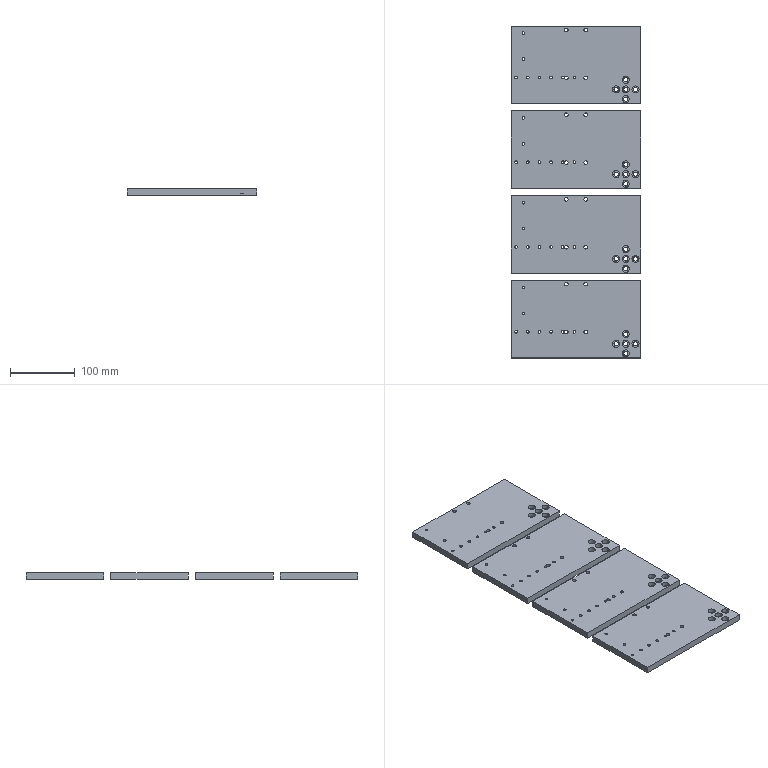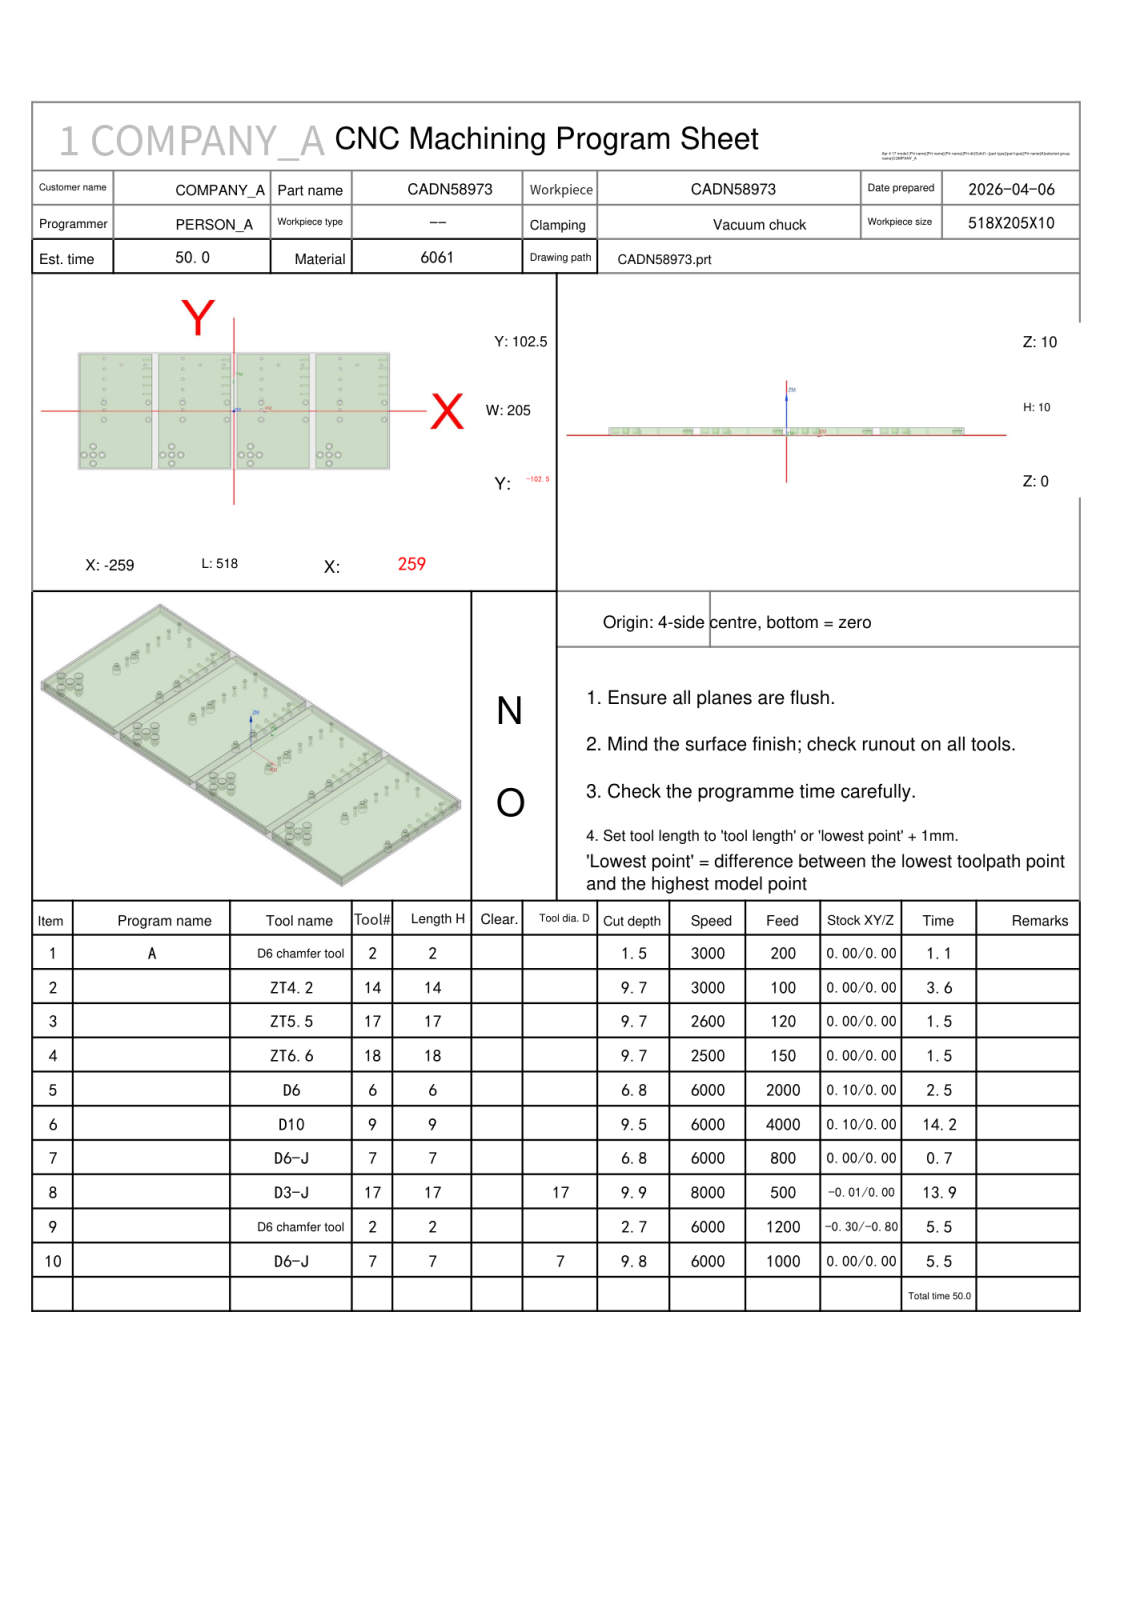NC program | NX | posted by the shop | part box 200 x 513 x 10 mm
Lines 1768 to 2551 of 10035:
N8 T17 M06
(D3-J  D=3. R=0. H=17 ce=-0.01 di=0.00)
G00 G90 G54 X-216.146 Y1.994 M03 S8000
G43 H17 Z30.
M08
Z10.5
G01 X-216.074 Y1.972 Z10.496 F500.
X-215.926 Z10.488
X-215.757 Y2.024 Z10.479
X-215.613 Y2.128 Z10.47
X-215.509 Y2.272 Z10.46
X-215.457 Y2.441 Z10.451
Y2.589 Z10.443
X-215.509 Y2.758 Z10.434
X-215.613 Y2.902 Z10.425
X-215.757 Y3.006 Z10.416
X-215.926 Y3.058 Z10.406
X-216.074 Z10.398
X-216.235 Y3.01 Z10.39
X-216.375 Y2.915 Z10.381
X-216.478 Y2.782 Z10.372
X-216.537 Y2.624 Z10.363
X-216.543 Y2.441 Z10.354
X-216.491 Y2.272 Z10.344
X-216.387 Y2.128 Z10.335
X-216.243 Y2.024 Z10.326
X-216.074 Y1.972 Z10.316
X-215.926 Z10.309
X-215.757 Y2.024 Z10.299
X-215.613 Y2.128 Z10.29
X-215.509 Y2.272 Z10.281
X-215.457 Y2.441 Z10.271
Y2.589 Z10.264
X-215.509 Y2.758 Z10.254
X-215.613 Y2.902 Z10.245
X-215.757 Y3.006 Z10.236
X-215.926 Y3.058 Z10.227
X-216.074 Z10.219
X-216.235 Y3.01 Z10.21
X-216.375 Y2.915 Z10.201
X-216.478 Y2.782 Z10.192
X-216.537 Y2.624 Z10.184
X-216.543 Y2.441 Z10.174
X-216.491 Y2.272 Z10.165
X-216.387 Y2.128 Z10.155
X-216.243 Y2.024 Z10.146
X-216.074 Y1.972 Z10.137
X-215.926 Z10.129
X-215.757 Y2.024 Z10.12
X-215.613 Y2.128 Z10.11
X-215.509 Y2.272 Z10.101
X-215.457 Y2.441 Z10.092
Y2.589 Z10.084
X-215.509 Y2.758 Z10.075
X-215.613 Y2.902 Z10.066
X-215.757 Y3.006 Z10.056
X-215.926 Y3.058 Z10.047
X-216.074 Z10.039
X-216.235 Y3.01 Z10.03
X-216.375 Y2.915 Z10.022
X-216.478 Y2.782 Z10.013
X-216.537 Y2.624 Z10.004
X-216.542 Y2.55 Z10.
G41 D17
X-216.577 Y2.515
G03 X-216. Y1.938 Z9.925 I.577 J0.0
X-215.423 Y2.515 Z9.851 I0.0 J.577
X-216. Y3.092 Z9.776 I-.577 J0.0
X-216.577 Y2.515 Z9.702 I0.0 J-.577
X-216. Y1.938 Z9.627 I.577 J0.0
X-215.423 Y2.515 Z9.552 I0.0 J.577
X-216. Y3.092 Z9.478 I-.577 J0.0
X-216.577 Y2.515 Z9.403 I0.0 J-.577
X-216. Y1.938 Z9.328 I.577 J0.0
X-215.423 Y2.515 Z9.254 I0.0 J.577
X-216. Y3.092 Z9.179 I-.577 J0.0
X-216.577 Y2.515 Z9.105 I0.0 J-.577
X-216. Y1.938 Z9.03 I.577 J0.0
X-215.423 Y2.515 Z8.955 I0.0 J.577
X-216. Y3.092 Z8.881 I-.577 J0.0
X-216.577 Y2.515 Z8.806 I0.0 J-.577
X-216. Y1.938 Z8.731 I.577 J0.0
X-215.423 Y2.515 Z8.657 I0.0 J.577
X-216. Y3.092 Z8.582 I-.577 J0.0
X-216.577 Y2.515 Z8.508 I0.0 J-.577
X-216. Y1.938 Z8.433 I.577 J0.0
X-215.423 Y2.515 Z8.358 I0.0 J.577
X-216. Y3.092 Z8.284 I-.577 J0.0
X-216.577 Y2.515 Z8.209 I0.0 J-.577
X-216. Y1.938 Z8.134 I.577 J0.0
X-215.423 Y2.515 Z8.06 I0.0 J.577
X-216. Y3.092 Z7.985 I-.577 J0.0
X-216.577 Y2.515 Z7.911 I0.0 J-.577
X-216. Y1.938 Z7.836 I.577 J0.0
X-215.423 Y2.515 Z7.761 I0.0 J.577
X-216. Y3.092 Z7.687 I-.577 J0.0
X-216.577 Y2.515 Z7.612 I0.0 J-.577
X-216. Y1.938 Z7.538 I.577 J0.0
X-215.423 Y2.515 Z7.463 I0.0 J.577
X-216. Y3.092 Z7.388 I-.577 J0.0
X-216.577 Y2.515 Z7.314 I0.0 J-.577
X-216. Y1.938 Z7.239 I.577 J0.0
X-215.423 Y2.515 Z7.164 I0.0 J.577
X-216. Y3.092 Z7.09 I-.577 J0.0
X-216.577 Y2.515 Z7.015 I0.0 J-.577
X-216. Y1.938 Z6.941 I.577 J0.0
X-215.423 Y2.515 Z6.866 I0.0 J.577
X-216. Y3.092 Z6.791 I-.577 J0.0
X-216.577 Y2.515 Z6.717 I0.0 J-.577
X-216. Y1.938 Z6.642 I.577 J0.0
X-215.423 Y2.515 Z6.567 I0.0 J.577
X-216. Y3.092 Z6.493 I-.577 J0.0
X-216.577 Y2.515 Z6.418 I0.0 J-.577
X-216. Y1.938 Z6.344 I.577 J0.0
X-215.423 Y2.515 Z6.269 I0.0 J.577
X-216. Y3.092 Z6.194 I-.577 J0.0
X-216.577 Y2.515 Z6.12 I0.0 J-.577
X-216. Y1.938 Z6.045 I.577 J0.0
X-215.423 Y2.515 Z5.97 I0.0 J.577
X-216. Y3.092 Z5.896 I-.577 J0.0
X-216.577 Y2.515 Z5.821 I0.0 J-.577
X-216. Y1.938 Z5.747 I.577 J0.0
X-215.423 Y2.515 Z5.672 I0.0 J.577
X-216. Y3.092 Z5.597 I-.577 J0.0
X-216.577 Y2.515 Z5.523 I0.0 J-.577
X-216. Y1.938 Z5.448 I.577 J0.0
X-215.423 Y2.515 Z5.373 I0.0 J.577
X-216. Y3.092 Z5.299 I-.577 J0.0
X-216.577 Y2.515 Z5.224 I0.0 J-.577
X-216. Y1.938 Z5.15 I.577 J0.0
X-215.423 Y2.515 Z5.075 I0.0 J.577
X-216. Y3.092 Z5. I-.577 J0.0
X-216.577 Y2.515 Z4.926 I0.0 J-.577
X-216. Y1.938 Z4.851 I.577 J0.0
X-215.423 Y2.515 Z4.777 I0.0 J.577
X-216. Y3.092 Z4.702 I-.577 J0.0
X-216.577 Y2.515 Z4.627 I0.0 J-.577
X-216. Y1.938 Z4.553 I.577 J0.0
X-215.423 Y2.515 Z4.478 I0.0 J.577
X-216. Y3.092 Z4.403 I-.577 J0.0
X-216.577 Y2.515 Z4.329 I0.0 J-.577
X-216. Y1.938 Z4.254 I.577 J0.0
X-215.423 Y2.515 Z4.18 I0.0 J.577
X-216. Y3.092 Z4.105 I-.577 J0.0
X-216.577 Y2.515 Z4.03 I0.0 J-.577
X-216. Y1.938 Z3.956 I.577 J0.0
X-215.423 Y2.515 Z3.881 I0.0 J.577
X-216. Y3.092 Z3.806 I-.577 J0.0
X-216.577 Y2.515 Z3.732 I0.0 J-.577
X-216. Y1.938 Z3.657 I.577 J0.0
X-215.423 Y2.515 Z3.583 I0.0 J.577
X-216. Y3.092 Z3.508 I-.577 J0.0
X-216.577 Y2.515 Z3.433 I0.0 J-.577
X-216. Y1.938 Z3.359 I.577 J0.0
X-215.423 Y2.515 Z3.284 I0.0 J.577
X-216. Y3.092 Z3.209 I-.577 J0.0
X-216.577 Y2.515 Z3.135 I0.0 J-.577
X-216. Y1.938 Z3.06 I.577 J0.0
X-215.423 Y2.515 Z2.986 I0.0 J.577
X-216. Y3.092 Z2.911 I-.577 J0.0
X-216.577 Y2.515 Z2.836 I0.0 J-.577
X-216. Y1.938 Z2.762 I.577 J0.0
X-215.423 Y2.515 Z2.687 I0.0 J.577
X-216. Y3.092 Z2.613 I-.577 J0.0
X-216.577 Y2.515 Z2.538 I0.0 J-.577
X-216. Y1.938 Z2.463 I.577 J0.0
X-215.423 Y2.515 Z2.389 I0.0 J.577
X-216. Y3.092 Z2.314 I-.577 J0.0
X-216.577 Y2.515 Z2.239 I0.0 J-.577
X-216. Y1.938 Z2.165 I.577 J0.0
X-215.423 Y2.515 Z2.09 I0.0 J.577
X-216. Y3.092 Z2.016 I-.577 J0.0
X-216.577 Y2.515 Z1.941 I0.0 J-.577
X-216. Y1.938 Z1.866 I.577 J0.0
X-215.423 Y2.515 Z1.792 I0.0 J.577
X-216. Y3.092 Z1.717 I-.577 J0.0
X-216.577 Y2.515 Z1.642 I0.0 J-.577
X-216. Y1.938 Z1.568 I.577 J0.0
X-215.423 Y2.515 Z1.493 I0.0 J.577
X-216. Y3.092 Z1.419 I-.577 J0.0
X-216.577 Y2.515 Z1.344 I0.0 J-.577
X-216. Y1.938 Z1.269 I.577 J0.0
X-215.423 Y2.515 Z1.195 I0.0 J.577
X-216. Y3.092 Z1.12 I-.577 J0.0
X-216.577 Y2.515 Z1.045 I0.0 J-.577
X-216. Y1.938 Z.971 I.577 J0.0
X-215.423 Y2.515 Z.896 I0.0 J.577
X-216. Y3.092 Z.822 I-.577 J0.0
X-216.577 Y2.515 Z.747 I0.0 J-.577
X-216. Y1.938 Z.672 I.577 J0.0
X-215.423 Y2.515 Z.598 I0.0 J.577
X-216. Y3.092 Z.523 I-.577 J0.0
X-216.577 Y2.515 Z.448 I0.0 J-.577
X-216. Y1.938 Z.374 I.577 J0.0
X-215.423 Y2.515 Z.299 I0.0 J.577
X-216. Y3.092 Z.225 I-.577 J0.0
X-216.577 Y2.515 Z.15 I0.0 J-.577
X-216. Y1.938 I.577 J0.0
X-215.423 Y2.515 I0.0 J.577
X-216. Y3.092 I-.577 J0.0
X-216.577 Y2.515 I0.0 J-.577
X-216.444 Y2.146 I.577 J0.0
G01 X-216.424 Y2.127
X-216.396 Y2.124
X-216.373 Y2.14
G40 X-216.335 Y2.172
Z1.15
G00 Z30.
X-216.144 Y37.994
Z10.5
G01 X-216.074 Y37.972 Z10.496
X-215.926 Z10.488
X-215.757 Y38.024 Z10.479
X-215.613 Y38.128 Z10.47
X-215.509 Y38.272 Z10.461
X-215.457 Y38.441 Z10.451
Y38.589 Z10.444
X-215.481 Y38.692 Z10.438
X-215.525 Y38.788 Z10.432
X-215.615 Y38.905 Z10.425
X-215.758 Y39.007 Z10.416
X-215.926 Y39.058 Z10.406
X-216.074 Z10.399
X-216.235 Y39.01 Z10.39
X-216.375 Y38.915 Z10.381
X-216.478 Y38.782 Z10.372
X-216.537 Y38.624 Z10.363
X-216.543 Y38.441 Z10.354
X-216.491 Y38.272 Z10.344
X-216.387 Y38.128 Z10.335
X-216.243 Y38.024 Z10.326
X-216.074 Y37.972 Z10.316
X-215.926 Z10.309
X-215.757 Y38.024 Z10.299
X-215.613 Y38.128 Z10.29
X-215.509 Y38.272 Z10.281
X-215.457 Y38.441 Z10.272
Y38.589 Z10.264
X-215.481 Y38.692 Z10.258
X-215.525 Y38.788 Z10.253
X-215.615 Y38.905 Z10.245
X-215.758 Y39.007 Z10.236
X-215.926 Y39.058 Z10.227
X-216.074 Z10.219
X-216.235 Y39.01 Z10.21
X-216.375 Y38.915 Z10.201
X-216.478 Y38.782 Z10.192
X-216.537 Y38.624 Z10.184
X-216.543 Y38.441 Z10.174
X-216.491 Y38.272 Z10.165
X-216.387 Y38.128 Z10.155
X-216.243 Y38.024 Z10.146
X-216.074 Y37.972 Z10.137
X-215.926 Z10.129
X-215.757 Y38.024 Z10.12
X-215.613 Y38.128 Z10.11
X-215.509 Y38.272 Z10.101
X-215.457 Y38.441 Z10.092
Y38.589 Z10.084
X-215.481 Y38.692 Z10.079
X-215.525 Y38.788 Z10.073
X-215.615 Y38.905 Z10.065
X-215.758 Y39.007 Z10.056
X-215.926 Y39.058 Z10.047
X-216.074 Z10.039
X-216.235 Y39.01 Z10.03
X-216.375 Y38.915 Z10.022
X-216.478 Y38.782 Z10.013
X-216.537 Y38.624 Z10.004
X-216.542 Y38.55 Z10.
G41 D17
X-216.577 Y38.515
G03 X-216. Y37.938 Z9.925 I.577 J0.0
X-215.423 Y38.515 Z9.851 I0.0 J.577
X-215.543 Y38.867 Z9.82 I-.577 J0.0
X-216. Y39.092 Z9.776 I-.457 J-.352
X-216.577 Y38.515 Z9.702 I0.0 J-.577
X-216. Y37.938 Z9.627 I.577 J0.0
X-215.423 Y38.515 Z9.552 I0.0 J.577
X-215.543 Y38.867 Z9.521 I-.577 J0.0
X-216. Y39.092 Z9.478 I-.457 J-.352
X-216.577 Y38.515 Z9.403 I0.0 J-.577
X-216. Y37.938 Z9.328 I.577 J0.0
X-215.423 Y38.515 Z9.254 I0.0 J.577
X-215.543 Y38.867 Z9.223 I-.577 J0.0
X-216. Y39.092 Z9.179 I-.457 J-.352
X-216.577 Y38.515 Z9.105 I0.0 J-.577
X-216. Y37.938 Z9.03 I.577 J0.0
X-215.423 Y38.515 Z8.955 I0.0 J.577
X-215.543 Y38.867 Z8.924 I-.577 J0.0
X-216. Y39.092 Z8.881 I-.457 J-.352
X-216.577 Y38.515 Z8.806 I0.0 J-.577
X-216. Y37.938 Z8.731 I.577 J0.0
X-215.423 Y38.515 Z8.657 I0.0 J.577
X-215.543 Y38.867 Z8.626 I-.577 J0.0
X-216. Y39.092 Z8.582 I-.457 J-.352
X-216.577 Y38.515 Z8.508 I0.0 J-.577
X-216. Y37.938 Z8.433 I.577 J0.0
X-215.423 Y38.515 Z8.358 I0.0 J.577
X-215.543 Y38.867 Z8.327 I-.577 J0.0
X-216. Y39.092 Z8.284 I-.457 J-.352
X-216.577 Y38.515 Z8.209 I0.0 J-.577
X-216. Y37.938 Z8.134 I.577 J0.0
X-215.423 Y38.515 Z8.06 I0.0 J.577
X-215.543 Y38.867 Z8.029 I-.577 J0.0
X-216. Y39.092 Z7.985 I-.457 J-.352
X-216.577 Y38.515 Z7.911 I0.0 J-.577
X-216. Y37.938 Z7.836 I.577 J0.0
X-215.423 Y38.515 Z7.761 I0.0 J.577
X-215.543 Y38.867 Z7.73 I-.577 J0.0
X-216. Y39.092 Z7.687 I-.457 J-.352
X-216.577 Y38.515 Z7.612 I0.0 J-.577
X-216. Y37.938 Z7.538 I.577 J0.0
X-215.423 Y38.515 Z7.463 I0.0 J.577
X-215.543 Y38.867 Z7.432 I-.577 J0.0
X-216. Y39.092 Z7.388 I-.457 J-.352
X-216.577 Y38.515 Z7.314 I0.0 J-.577
X-216. Y37.938 Z7.239 I.577 J0.0
X-215.423 Y38.515 Z7.164 I0.0 J.577
X-215.543 Y38.867 Z7.133 I-.577 J0.0
X-216. Y39.092 Z7.09 I-.457 J-.352
X-216.577 Y38.515 Z7.015 I0.0 J-.577
X-216. Y37.938 Z6.941 I.577 J0.0
X-215.423 Y38.515 Z6.866 I0.0 J.577
X-215.543 Y38.867 Z6.835 I-.577 J0.0
X-216. Y39.092 Z6.791 I-.457 J-.352
X-216.577 Y38.515 Z6.717 I0.0 J-.577
X-216. Y37.938 Z6.642 I.577 J0.0
X-215.423 Y38.515 Z6.567 I0.0 J.577
X-215.543 Y38.867 Z6.536 I-.577 J0.0
X-216. Y39.092 Z6.493 I-.457 J-.352
X-216.577 Y38.515 Z6.418 I0.0 J-.577
X-216. Y37.938 Z6.344 I.577 J0.0
X-215.423 Y38.515 Z6.269 I0.0 J.577
X-215.543 Y38.867 Z6.238 I-.577 J0.0
X-216. Y39.092 Z6.194 I-.457 J-.352
X-216.577 Y38.515 Z6.12 I0.0 J-.577
X-216. Y37.938 Z6.045 I.577 J0.0
X-215.423 Y38.515 Z5.97 I0.0 J.577
X-215.543 Y38.867 Z5.939 I-.577 J0.0
X-216. Y39.092 Z5.896 I-.457 J-.352
X-216.577 Y38.515 Z5.821 I0.0 J-.577
X-216. Y37.938 Z5.747 I.577 J0.0
X-215.423 Y38.515 Z5.672 I0.0 J.577
X-215.543 Y38.867 Z5.641 I-.577 J0.0
X-216. Y39.092 Z5.597 I-.457 J-.352
X-216.577 Y38.515 Z5.523 I0.0 J-.577
X-216. Y37.938 Z5.448 I.577 J0.0
X-215.423 Y38.515 Z5.373 I0.0 J.577
X-215.543 Y38.867 Z5.342 I-.577 J0.0
X-216. Y39.092 Z5.299 I-.457 J-.352
X-216.577 Y38.515 Z5.224 I0.0 J-.577
X-216. Y37.938 Z5.15 I.577 J0.0
X-215.423 Y38.515 Z5.075 I0.0 J.577
X-215.543 Y38.867 Z5.044 I-.577 J0.0
X-216. Y39.092 Z5. I-.457 J-.352
X-216.577 Y38.515 Z4.926 I0.0 J-.577
X-216. Y37.938 Z4.851 I.577 J0.0
X-215.423 Y38.515 Z4.777 I0.0 J.577
X-215.543 Y38.867 Z4.745 I-.577 J0.0
X-216. Y39.092 Z4.702 I-.457 J-.352
X-216.577 Y38.515 Z4.627 I0.0 J-.577
X-216. Y37.938 Z4.553 I.577 J0.0
X-215.423 Y38.515 Z4.478 I0.0 J.577
X-215.543 Y38.867 Z4.447 I-.577 J0.0
X-216. Y39.092 Z4.403 I-.457 J-.352
X-216.577 Y38.515 Z4.329 I0.0 J-.577
X-216. Y37.938 Z4.254 I.577 J0.0
X-215.423 Y38.515 Z4.18 I0.0 J.577
X-215.543 Y38.867 Z4.148 I-.577 J0.0
X-216. Y39.092 Z4.105 I-.457 J-.352
X-216.577 Y38.515 Z4.03 I0.0 J-.577
X-216. Y37.938 Z3.956 I.577 J0.0
X-215.423 Y38.515 Z3.881 I0.0 J.577
X-215.543 Y38.867 Z3.85 I-.577 J0.0
X-216. Y39.092 Z3.806 I-.457 J-.352
X-216.577 Y38.515 Z3.732 I0.0 J-.577
X-216. Y37.938 Z3.657 I.577 J0.0
X-215.423 Y38.515 Z3.583 I0.0 J.577
X-215.543 Y38.867 Z3.551 I-.577 J0.0
X-216. Y39.092 Z3.508 I-.457 J-.352
X-216.577 Y38.515 Z3.433 I0.0 J-.577
X-216. Y37.938 Z3.359 I.577 J0.0
X-215.423 Y38.515 Z3.284 I0.0 J.577
X-215.543 Y38.867 Z3.253 I-.577 J0.0
X-216. Y39.092 Z3.209 I-.457 J-.352
X-216.577 Y38.515 Z3.135 I0.0 J-.577
X-216. Y37.938 Z3.06 I.577 J0.0
X-215.423 Y38.515 Z2.986 I0.0 J.577
X-215.543 Y38.867 Z2.954 I-.577 J0.0
X-216. Y39.092 Z2.911 I-.457 J-.352
X-216.577 Y38.515 Z2.836 I0.0 J-.577
X-216. Y37.938 Z2.762 I.577 J0.0
X-215.423 Y38.515 Z2.687 I0.0 J.577
X-215.543 Y38.867 Z2.656 I-.577 J0.0
X-216. Y39.092 Z2.613 I-.457 J-.352
X-216.577 Y38.515 Z2.538 I0.0 J-.577
X-216. Y37.938 Z2.463 I.577 J0.0
X-215.423 Y38.515 Z2.389 I0.0 J.577
X-215.543 Y38.867 Z2.357 I-.577 J0.0
X-216. Y39.092 Z2.314 I-.457 J-.352
X-216.577 Y38.515 Z2.239 I0.0 J-.577
X-216. Y37.938 Z2.165 I.577 J0.0
X-215.423 Y38.515 Z2.09 I0.0 J.577
X-215.543 Y38.867 Z2.059 I-.577 J0.0
X-216. Y39.092 Z2.016 I-.457 J-.352
X-216.577 Y38.515 Z1.941 I0.0 J-.577
X-216. Y37.938 Z1.866 I.577 J0.0
X-215.423 Y38.515 Z1.792 I0.0 J.577
X-215.543 Y38.867 Z1.76 I-.577 J0.0
X-216. Y39.092 Z1.717 I-.457 J-.352
X-216.577 Y38.515 Z1.642 I0.0 J-.577
X-216. Y37.938 Z1.568 I.577 J0.0
X-215.423 Y38.515 Z1.493 I0.0 J.577
X-215.543 Y38.867 Z1.462 I-.577 J0.0
X-216. Y39.092 Z1.419 I-.457 J-.352
X-216.577 Y38.515 Z1.344 I0.0 J-.577
X-216. Y37.938 Z1.269 I.577 J0.0
X-215.423 Y38.515 Z1.195 I0.0 J.577
X-215.543 Y38.867 Z1.164 I-.577 J0.0
X-216. Y39.092 Z1.12 I-.457 J-.352
X-216.577 Y38.515 Z1.045 I0.0 J-.577
X-216. Y37.938 Z.971 I.577 J0.0
X-215.423 Y38.515 Z.896 I0.0 J.577
X-215.543 Y38.867 Z.865 I-.577 J0.0
X-216. Y39.092 Z.822 I-.457 J-.352
X-216.577 Y38.515 Z.747 I0.0 J-.577
X-216. Y37.938 Z.672 I.577 J0.0
X-215.423 Y38.515 Z.598 I0.0 J.577
X-215.543 Y38.867 Z.567 I-.577 J0.0
X-216. Y39.092 Z.523 I-.457 J-.352
X-216.577 Y38.515 Z.448 I0.0 J-.577
X-216. Y37.938 Z.374 I.577 J0.0
X-215.423 Y38.515 Z.299 I0.0 J.577
X-215.543 Y38.867 Z.268 I-.577 J0.0
X-216. Y39.092 Z.225 I-.457 J-.352
X-216.577 Y38.515 Z.15 I0.0 J-.577
X-216. Y37.938 I.577 J0.0
X-215.423 Y38.515 I0.0 J.577
X-216. Y39.092 I-.577 J0.0
X-216.577 Y38.515 I0.0 J-.577
X-216.444 Y38.146 I.577 J0.0
G01 X-216.424 Y38.127
X-216.396 Y38.124
X-216.373 Y38.14
G40 X-216.335 Y38.172
Z1.15
G00 Z30.
X-216.146 Y55.994
Z10.5
G01 X-216.074 Y55.972 Z10.496
X-215.926 Z10.488
X-215.757 Y56.024 Z10.479
X-215.613 Y56.128 Z10.47
X-215.509 Y56.272 Z10.46
X-215.457 Y56.441 Z10.451
Y56.589 Z10.443
X-215.509 Y56.758 Z10.434
X-215.613 Y56.902 Z10.425
X-215.757 Y57.006 Z10.416
X-215.926 Y57.058 Z10.406
X-216.074 Z10.398
X-216.235 Y57.01 Z10.39
X-216.375 Y56.915 Z10.381
X-216.478 Y56.782 Z10.372
X-216.537 Y56.624 Z10.363
X-216.543 Y56.441 Z10.354
X-216.491 Y56.272 Z10.344
X-216.387 Y56.128 Z10.335
X-216.243 Y56.024 Z10.326
X-216.074 Y55.972 Z10.316
X-215.926 Z10.309
X-215.757 Y56.024 Z10.299
X-215.613 Y56.128 Z10.29
X-215.509 Y56.272 Z10.281
X-215.457 Y56.441 Z10.271
Y56.589 Z10.264
X-215.509 Y56.758 Z10.254
X-215.613 Y56.902 Z10.245
X-215.757 Y57.006 Z10.236
X-215.926 Y57.058 Z10.227
X-216.074 Z10.219
X-216.235 Y57.01 Z10.21
X-216.375 Y56.915 Z10.201
X-216.478 Y56.782 Z10.192
X-216.537 Y56.624 Z10.184
X-216.543 Y56.441 Z10.174
X-216.491 Y56.272 Z10.165
X-216.387 Y56.128 Z10.155
X-216.243 Y56.024 Z10.146
X-216.074 Y55.972 Z10.137
X-215.926 Z10.129
X-215.757 Y56.024 Z10.12
X-215.613 Y56.128 Z10.11
X-215.509 Y56.272 Z10.101
X-215.457 Y56.441 Z10.092
Y56.589 Z10.084
X-215.509 Y56.758 Z10.075
X-215.613 Y56.902 Z10.066
X-215.757 Y57.006 Z10.056
X-215.926 Y57.058 Z10.047
X-216.074 Z10.039
X-216.235 Y57.01 Z10.03
X-216.375 Y56.915 Z10.022
X-216.478 Y56.782 Z10.013
X-216.537 Y56.624 Z10.004
X-216.542 Y56.55 Z10.
G41 D17
X-216.577 Y56.515
G03 X-216. Y55.938 Z9.925 I.577 J0.0
X-215.423 Y56.515 Z9.851 I0.0 J.577
X-216. Y57.092 Z9.776 I-.577 J0.0
X-216.577 Y56.515 Z9.702 I0.0 J-.577
X-216. Y55.938 Z9.627 I.577 J0.0
X-215.423 Y56.515 Z9.552 I0.0 J.577
X-216. Y57.092 Z9.478 I-.577 J0.0
X-216.577 Y56.515 Z9.403 I0.0 J-.577
X-216. Y55.938 Z9.328 I.577 J0.0
X-215.423 Y56.515 Z9.254 I0.0 J.577
X-216. Y57.092 Z9.179 I-.577 J0.0
X-216.577 Y56.515 Z9.105 I0.0 J-.577
X-216. Y55.938 Z9.03 I.577 J0.0
X-215.423 Y56.515 Z8.955 I0.0 J.577
X-216. Y57.092 Z8.881 I-.577 J0.0
X-216.577 Y56.515 Z8.806 I0.0 J-.577
X-216. Y55.938 Z8.731 I.577 J0.0
X-215.423 Y56.515 Z8.657 I0.0 J.577
X-216. Y57.092 Z8.582 I-.577 J0.0
X-216.577 Y56.515 Z8.508 I0.0 J-.577
X-216. Y55.938 Z8.433 I.577 J0.0
X-215.423 Y56.515 Z8.358 I0.0 J.577
X-216. Y57.092 Z8.284 I-.577 J0.0
X-216.577 Y56.515 Z8.209 I0.0 J-.577
X-216. Y55.938 Z8.134 I.577 J0.0
X-215.423 Y56.515 Z8.06 I0.0 J.577
X-216. Y57.092 Z7.985 I-.577 J0.0
X-216.577 Y56.515 Z7.911 I0.0 J-.577
X-216. Y55.938 Z7.836 I.577 J0.0
X-215.423 Y56.515 Z7.761 I0.0 J.577
X-216. Y57.092 Z7.687 I-.577 J0.0
X-216.577 Y56.515 Z7.612 I0.0 J-.577
X-216. Y55.938 Z7.538 I.577 J0.0
X-215.423 Y56.515 Z7.463 I0.0 J.577
X-216. Y57.092 Z7.388 I-.577 J0.0
X-216.577 Y56.515 Z7.314 I0.0 J-.577
X-216. Y55.938 Z7.239 I.577 J0.0
X-215.423 Y56.515 Z7.164 I0.0 J.577
X-216. Y57.092 Z7.09 I-.577 J0.0
X-216.577 Y56.515 Z7.015 I0.0 J-.577
X-216. Y55.938 Z6.941 I.577 J0.0
X-215.423 Y56.515 Z6.866 I0.0 J.577
X-216. Y57.092 Z6.791 I-.577 J0.0
X-216.577 Y56.515 Z6.717 I0.0 J-.577
X-216. Y55.938 Z6.642 I.577 J0.0
X-215.423 Y56.515 Z6.567 I0.0 J.577
X-216. Y57.092 Z6.493 I-.577 J0.0
X-216.577 Y56.515 Z6.418 I0.0 J-.577
X-216. Y55.938 Z6.344 I.577 J0.0
X-215.423 Y56.515 Z6.269 I0.0 J.577
X-216. Y57.092 Z6.194 I-.577 J0.0
X-216.577 Y56.515 Z6.12 I0.0 J-.577
X-216. Y55.938 Z6.045 I.577 J0.0
X-215.423 Y56.515 Z5.97 I0.0 J.577
X-216. Y57.092 Z5.896 I-.577 J0.0
X-216.577 Y56.515 Z5.821 I0.0 J-.577
X-216. Y55.938 Z5.747 I.577 J0.0
X-215.423 Y56.515 Z5.672 I0.0 J.577
X-216. Y57.092 Z5.597 I-.577 J0.0
X-216.577 Y56.515 Z5.523 I0.0 J-.577
X-216. Y55.938 Z5.448 I.577 J0.0
X-215.423 Y56.515 Z5.373 I0.0 J.577
X-216. Y57.092 Z5.299 I-.577 J0.0
X-216.577 Y56.515 Z5.224 I0.0 J-.577
X-216. Y55.938 Z5.15 I.577 J0.0
X-215.423 Y56.515 Z5.075 I0.0 J.577
X-216. Y57.092 Z5. I-.577 J0.0
X-216.577 Y56.515 Z4.926 I0.0 J-.577
X-216. Y55.938 Z4.851 I.577 J0.0
X-215.423 Y56.515 Z4.777 I0.0 J.577
X-216. Y57.092 Z4.702 I-.577 J0.0
X-216.577 Y56.515 Z4.627 I0.0 J-.577
X-216. Y55.938 Z4.553 I.577 J0.0
X-215.423 Y56.515 Z4.478 I0.0 J.577
X-216. Y57.092 Z4.403 I-.577 J0.0
X-216.577 Y56.515 Z4.329 I0.0 J-.577
X-216. Y55.938 Z4.254 I.577 J0.0
X-215.423 Y56.515 Z4.18 I0.0 J.577
X-216. Y57.092 Z4.105 I-.577 J0.0
X-216.577 Y56.515 Z4.03 I0.0 J-.577
X-216. Y55.938 Z3.956 I.577 J0.0
X-215.423 Y56.515 Z3.881 I0.0 J.577
X-216. Y57.092 Z3.806 I-.577 J0.0
X-216.577 Y56.515 Z3.732 I0.0 J-.577
X-216. Y55.938 Z3.657 I.577 J0.0
X-215.423 Y56.515 Z3.583 I0.0 J.577
X-216. Y57.092 Z3.508 I-.577 J0.0
X-216.577 Y56.515 Z3.433 I0.0 J-.577
X-216. Y55.938 Z3.359 I.577 J0.0
X-215.423 Y56.515 Z3.284 I0.0 J.577
X-216. Y57.092 Z3.209 I-.577 J0.0
X-216.577 Y56.515 Z3.135 I0.0 J-.577
X-216. Y55.938 Z3.06 I.577 J0.0
X-215.423 Y56.515 Z2.986 I0.0 J.577
X-216. Y57.092 Z2.911 I-.577 J0.0
X-216.577 Y56.515 Z2.836 I0.0 J-.577
X-216. Y55.938 Z2.762 I.577 J0.0
X-215.423 Y56.515 Z2.687 I0.0 J.577
X-216. Y57.092 Z2.613 I-.577 J0.0
X-216.577 Y56.515 Z2.538 I0.0 J-.577
X-216. Y55.938 Z2.463 I.577 J0.0
X-215.423 Y56.515 Z2.389 I0.0 J.577
X-216. Y57.092 Z2.314 I-.577 J0.0
X-216.577 Y56.515 Z2.239 I0.0 J-.577
X-216. Y55.938 Z2.165 I.577 J0.0
X-215.423 Y56.515 Z2.09 I0.0 J.577
X-216. Y57.092 Z2.016 I-.577 J0.0
X-216.577 Y56.515 Z1.941 I0.0 J-.577
X-216. Y55.938 Z1.866 I.577 J0.0
X-215.423 Y56.515 Z1.792 I0.0 J.577
X-216. Y57.092 Z1.717 I-.577 J0.0
X-216.577 Y56.515 Z1.642 I0.0 J-.577
X-216. Y55.938 Z1.568 I.577 J0.0
X-215.423 Y56.515 Z1.493 I0.0 J.577
X-216. Y57.092 Z1.419 I-.577 J0.0
X-216.577 Y56.515 Z1.344 I0.0 J-.577
X-216. Y55.938 Z1.269 I.577 J0.0
X-215.423 Y56.515 Z1.195 I0.0 J.577
X-216. Y57.092 Z1.12 I-.577 J0.0
X-216.577 Y56.515 Z1.045 I0.0 J-.577
X-216. Y55.938 Z.971 I.577 J0.0
X-215.423 Y56.515 Z.896 I0.0 J.577
X-216. Y57.092 Z.822 I-.577 J0.0
X-216.577 Y56.515 Z.747 I0.0 J-.577
X-216. Y55.938 Z.672 I.577 J0.0
X-215.423 Y56.515 Z.598 I0.0 J.577
X-216. Y57.092 Z.523 I-.577 J0.0
X-216.577 Y56.515 Z.448 I0.0 J-.577
X-216. Y55.938 Z.374 I.577 J0.0
X-215.423 Y56.515 Z.299 I0.0 J.577
X-216. Y57.092 Z.225 I-.577 J0.0
X-216.577 Y56.515 Z.15 I0.0 J-.577
X-216. Y55.938 I.577 J0.0
X-215.423 Y56.515 I0.0 J.577
X-216. Y57.092 I-.577 J0.0
X-216.577 Y56.515 I0.0 J-.577
X-216.444 Y56.146 I.577 J0.0
G01 X-216.424 Y56.127
X-216.396 Y56.124
X-216.373 Y56.14
G40 X-216.335 Y56.172
Z1.15
G00 Z30.
X-216.521 Y74.661
Z10.5
G01 X-216.543 Y74.589 Z10.496
Y74.441 Z10.488
X-216.491 Y74.272 Z10.479
X-216.387 Y74.128 Z10.47
X-216.243 Y74.024 Z10.46
X-216.074 Y73.972 Z10.451
X-215.926 Z10.443
X-215.757 Y74.024 Z10.434
X-215.613 Y74.128 Z10.425
X-215.509 Y74.272 Z10.416
X-215.457 Y74.441 Z10.406
Y74.589 Z10.398
X-215.505 Y74.75 Z10.39
X-215.6 Y74.89 Z10.381
X-215.733 Y74.993 Z10.372
X-215.891 Y75.052 Z10.363
X-216.074 Y75.058 Z10.354
X-216.243 Y75.006 Z10.344
X-216.387 Y74.902 Z10.335
X-216.491 Y74.758 Z10.326
X-216.543 Y74.589 Z10.316
Y74.441 Z10.309
X-216.491 Y74.272 Z10.299
X-216.387 Y74.128 Z10.29
X-216.243 Y74.024 Z10.281
X-216.074 Y73.972 Z10.271
X-215.926 Z10.264
X-215.757 Y74.024 Z10.254
X-215.613 Y74.128 Z10.245
X-215.509 Y74.272 Z10.236
X-215.457 Y74.441 Z10.227
Y74.589 Z10.219
X-215.505 Y74.75 Z10.21
X-215.6 Y74.89 Z10.201
X-215.733 Y74.993 Z10.192
X-215.891 Y75.052 Z10.184
X-216.074 Y75.058 Z10.174
X-216.243 Y75.006 Z10.165
X-216.387 Y74.902 Z10.155
X-216.491 Y74.758 Z10.146
X-216.543 Y74.589 Z10.137
Y74.441 Z10.129
X-216.491 Y74.272 Z10.12
X-216.387 Y74.128 Z10.11
X-216.243 Y74.024 Z10.101
X-216.074 Y73.972 Z10.092
X-215.926 Z10.084
X-215.757 Y74.024 Z10.075
X-215.613 Y74.128 Z10.066
X-215.509 Y74.272 Z10.056
X-215.457 Y74.441 Z10.047
Y74.589 Z10.039
X-215.505 Y74.75 Z10.03
X-215.6 Y74.89 Z10.022
X-215.733 Y74.993 Z10.013
X-215.891 Y75.052 Z10.004
X-215.965 Y75.057 Z10.
G41 D17
X-216. Y75.092
G03 X-216.577 Y74.515 Z9.925 I0.0 J-.577
X-216. Y73.938 Z9.851 I.577 J0.0
X-215.423 Y74.515 Z9.776 I0.0 J.577
X-216. Y75.092 Z9.702 I-.577 J0.0
X-216.577 Y74.515 Z9.627 I0.0 J-.577
X-216. Y73.938 Z9.552 I.577 J0.0
X-215.423 Y74.515 Z9.478 I0.0 J.577
X-216. Y75.092 Z9.403 I-.577 J0.0
X-216.577 Y74.515 Z9.328 I0.0 J-.577
X-216. Y73.938 Z9.254 I.577 J0.0
X-215.423 Y74.515 Z9.179 I0.0 J.577
X-216. Y75.092 Z9.105 I-.577 J0.0
X-216.577 Y74.515 Z9.03 I0.0 J-.577
X-216. Y73.938 Z8.955 I.577 J0.0
X-215.423 Y74.515 Z8.881 I0.0 J.577
X-216. Y75.092 Z8.806 I-.577 J0.0
X-216.577 Y74.515 Z8.731 I0.0 J-.577
X-216. Y73.938 Z8.657 I.577 J0.0
X-215.423 Y74.515 Z8.582 I0.0 J.577
X-216. Y75.092 Z8.508 I-.577 J0.0
X-216.577 Y74.515 Z8.433 I0.0 J-.577
X-216. Y73.938 Z8.358 I.577 J0.0
X-215.423 Y74.515 Z8.284 I0.0 J.577
X-216. Y75.092 Z8.209 I-.577 J0.0
X-216.577 Y74.515 Z8.134 I0.0 J-.577
X-216. Y73.938 Z8.06 I.577 J0.0
X-215.423 Y74.515 Z7.985 I0.0 J.577
X-216. Y75.092 Z7.911 I-.577 J0.0
X-216.577 Y74.515 Z7.836 I0.0 J-.577
X-216. Y73.938 Z7.761 I.577 J0.0
X-215.423 Y74.515 Z7.687 I0.0 J.577
X-216. Y75.092 Z7.612 I-.577 J0.0
X-216.577 Y74.515 Z7.538 I0.0 J-.577
X-216. Y73.938 Z7.463 I.577 J0.0
X-215.423 Y74.515 Z7.388 I0.0 J.577
X-216. Y75.092 Z7.314 I-.577 J0.0
X-216.577 Y74.515 Z7.239 I0.0 J-.577
X-216. Y73.938 Z7.164 I.577 J0.0
X-215.423 Y74.515 Z7.09 I0.0 J.577
X-216. Y75.092 Z7.015 I-.577 J0.0
X-216.577 Y74.515 Z6.941 I0.0 J-.577
X-216. Y73.938 Z6.866 I.577 J0.0
X-215.423 Y74.515 Z6.791 I0.0 J.577
X-216. Y75.092 Z6.717 I-.577 J0.0
X-216.577 Y74.515 Z6.642 I0.0 J-.577
X-216. Y73.938 Z6.567 I.577 J0.0
X-215.423 Y74.515 Z6.493 I0.0 J.577
X-216. Y75.092 Z6.418 I-.577 J0.0
X-216.577 Y74.515 Z6.344 I0.0 J-.577
X-216. Y73.938 Z6.269 I.577 J0.0
X-215.423 Y74.515 Z6.194 I0.0 J.577
X-216. Y75.092 Z6.12 I-.577 J0.0
X-216.577 Y74.515 Z6.045 I0.0 J-.577
X-216. Y73.938 Z5.97 I.577 J0.0
X-215.423 Y74.515 Z5.896 I0.0 J.577
X-216. Y75.092 Z5.821 I-.577 J0.0
X-216.577 Y74.515 Z5.747 I0.0 J-.577
X-216. Y73.938 Z5.672 I.577 J0.0
X-215.423 Y74.515 Z5.597 I0.0 J.577
X-216. Y75.092 Z5.523 I-.577 J0.0
X-216.577 Y74.515 Z5.448 I0.0 J-.577
X-216. Y73.938 Z5.373 I.577 J0.0
X-215.423 Y74.515 Z5.299 I0.0 J.577
X-216. Y75.092 Z5.224 I-.577 J0.0
X-216.577 Y74.515 Z5.15 I0.0 J-.577
X-216. Y73.938 Z5.075 I.577 J0.0
X-215.423 Y74.515 Z5. I0.0 J.577
X-216. Y75.092 Z4.926 I-.577 J0.0
X-216.577 Y74.515 Z4.851 I0.0 J-.577
X-216. Y73.938 Z4.777 I.577 J0.0
X-215.423 Y74.515 Z4.702 I0.0 J.577